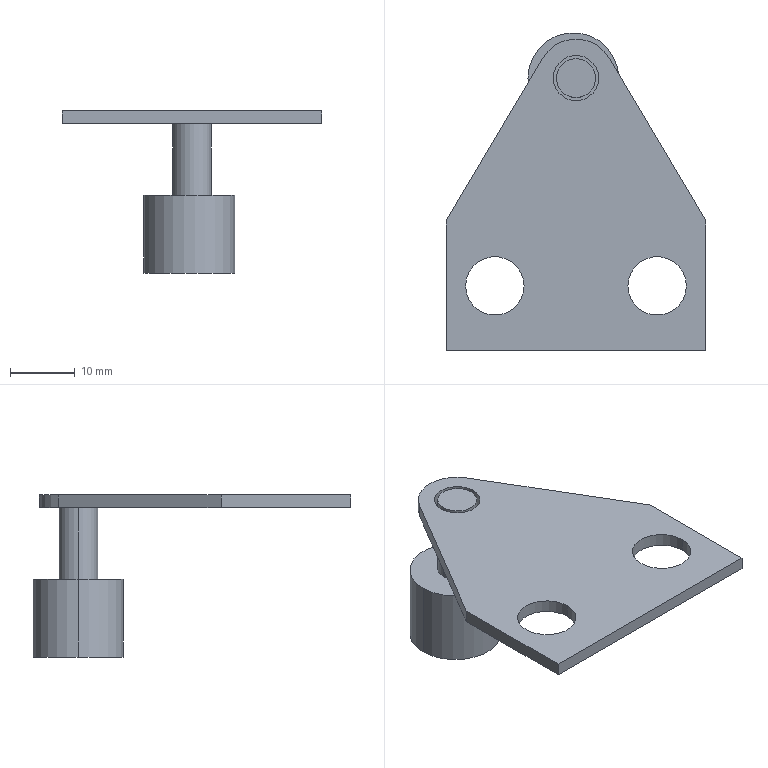Part | SolidWorks | features BaseBody 2 | 2 solids | 21 faces | box 40 x 49 x 25 mm | volume 4787 mm3 | cylinder 11 | plane 10 | commonest cylinder face diameters 9 x4 6 x2 7 x2 14 x2 12 x1
STEP:
#1=CARTESIAN_POINT('',(28.,10.,0.));
#2=VERTEX_POINT('',#1);
#3=CARTESIAN_POINT('',(37.,10.,0.));
#4=VERTEX_POINT('',#3);
#5=CARTESIAN_POINT('',(32.5,10.,0.));
#6=DIRECTION('',(0.,0.,1.));
#7=DIRECTION('',(1.,0.,0.));
#8=AXIS2_PLACEMENT_3D('',#5,#6,#7);
#9=CIRCLE('',#8,4.5);
#10=EDGE_CURVE('',#2,#4,#9,.T.);
#11=ORIENTED_EDGE('',*,*,#10,.F.);
#12=CARTESIAN_POINT('',(28.,10.,2.));
#13=VERTEX_POINT('',#12);
#14=CARTESIAN_POINT('',(28.,10.,0.));
#15=DIRECTION('',(0.,0.,1.));
#16=VECTOR('',#15,1000.);
#17=LINE('',#14,#16);
#18=EDGE_CURVE('',#2,#13,#17,.T.);
#19=ORIENTED_EDGE('',*,*,#18,.T.);
#20=CARTESIAN_POINT('',(37.,10.,2.));
#21=VERTEX_POINT('',#20);
#22=CARTESIAN_POINT('',(32.5,10.,2.));
#23=DIRECTION('',(0.,0.,1.));
#24=DIRECTION('',(1.,0.,0.));
#25=AXIS2_PLACEMENT_3D('',#22,#23,#24);
#26=CIRCLE('',#25,4.5);
#27=EDGE_CURVE('',#13,#21,#26,.T.);
#28=ORIENTED_EDGE('',*,*,#27,.T.);
#29=CARTESIAN_POINT('',(37.,10.,0.));
#30=DIRECTION('',(0.,0.,1.));
#31=VECTOR('',#30,1000.);
#32=LINE('',#29,#31);
#33=EDGE_CURVE('',#4,#21,#32,.T.);
#34=ORIENTED_EDGE('',*,*,#33,.F.);
#35=EDGE_LOOP('',(#11,#19,#28,#34));
#36=FACE_OUTER_BOUND('',#35,.T.);
#37=CARTESIAN_POINT('',(32.5,10.,0.));
#38=DIRECTION('',(0.,0.,1.));
#39=DIRECTION('',(1.,0.,0.));
#40=AXIS2_PLACEMENT_3D('',#37,#38,#39);
#41=CYLINDRICAL_SURFACE('',#40,4.5);
#42=ADVANCED_FACE('',(#36),#41,.F.);
#43=CARTESIAN_POINT('',(3.,10.,0.));
#44=VERTEX_POINT('',#43);
#45=CARTESIAN_POINT('',(12.,10.,0.));
#46=VERTEX_POINT('',#45);
#47=CARTESIAN_POINT('',(7.5,10.,0.));
#48=DIRECTION('',(0.,0.,1.));
#49=DIRECTION('',(1.,0.,0.));
#50=AXIS2_PLACEMENT_3D('',#47,#48,#49);
#51=CIRCLE('',#50,4.5);
#52=EDGE_CURVE('',#44,#46,#51,.T.);
#53=ORIENTED_EDGE('',*,*,#52,.F.);
#54=CARTESIAN_POINT('',(3.,10.,2.));
#55=VERTEX_POINT('',#54);
#56=CARTESIAN_POINT('',(3.,10.,0.));
#57=DIRECTION('',(0.,0.,1.));
#58=VECTOR('',#57,1000.);
#59=LINE('',#56,#58);
#60=EDGE_CURVE('',#44,#55,#59,.T.);
#61=ORIENTED_EDGE('',*,*,#60,.T.);
#62=CARTESIAN_POINT('',(12.,10.,2.));
#63=VERTEX_POINT('',#62);
#64=CARTESIAN_POINT('',(7.5,10.,2.));
#65=DIRECTION('',(0.,0.,1.));
#66=DIRECTION('',(1.,0.,0.));
#67=AXIS2_PLACEMENT_3D('',#64,#65,#66);
#68=CIRCLE('',#67,4.5);
#69=EDGE_CURVE('',#55,#63,#68,.T.);
#70=ORIENTED_EDGE('',*,*,#69,.T.);
#71=CARTESIAN_POINT('',(12.,10.,0.));
#72=DIRECTION('',(0.,0.,1.));
#73=VECTOR('',#72,1000.);
#74=LINE('',#71,#73);
#75=EDGE_CURVE('',#46,#63,#74,.T.);
#76=ORIENTED_EDGE('',*,*,#75,.F.);
#77=EDGE_LOOP('',(#53,#61,#70,#76));
#78=FACE_OUTER_BOUND('',#77,.T.);
#79=CARTESIAN_POINT('',(7.5,10.,0.));
#80=DIRECTION('',(0.,0.,1.));
#81=DIRECTION('',(1.,0.,0.));
#82=AXIS2_PLACEMENT_3D('',#79,#80,#81);
#83=CYLINDRICAL_SURFACE('',#82,4.5);
#84=ADVANCED_FACE('',(#78),#83,.F.);
#85=CARTESIAN_POINT('',(16.5,42.,0.));
#86=VERTEX_POINT('',#85);
#87=CARTESIAN_POINT('',(23.5,42.,0.));
#88=VERTEX_POINT('',#87);
#89=CARTESIAN_POINT('',(20.,42.,0.));
#90=DIRECTION('',(0.,0.,1.));
#91=DIRECTION('',(1.,0.,0.));
#92=AXIS2_PLACEMENT_3D('',#89,#90,#91);
#93=CIRCLE('',#92,3.5);
#94=EDGE_CURVE('',#86,#88,#93,.T.);
#95=ORIENTED_EDGE('',*,*,#94,.F.);
#96=CARTESIAN_POINT('',(16.5,42.,2.));
#97=VERTEX_POINT('',#96);
#98=CARTESIAN_POINT('',(16.5,42.,0.));
#99=DIRECTION('',(0.,0.,1.));
#100=VECTOR('',#99,1000.);
#101=LINE('',#98,#100);
#102=EDGE_CURVE('',#86,#97,#101,.T.);
#103=ORIENTED_EDGE('',*,*,#102,.T.);
#104=CARTESIAN_POINT('',(23.5,42.,2.));
#105=VERTEX_POINT('',#104);
#106=CARTESIAN_POINT('',(20.,42.,2.));
#107=DIRECTION('',(0.,0.,1.));
#108=DIRECTION('',(1.,0.,0.));
#109=AXIS2_PLACEMENT_3D('',#106,#107,#108);
#110=CIRCLE('',#109,3.5);
#111=EDGE_CURVE('',#97,#105,#110,.T.);
#112=ORIENTED_EDGE('',*,*,#111,.T.);
#113=CARTESIAN_POINT('',(23.5,42.,0.));
#114=DIRECTION('',(0.,0.,1.));
#115=VECTOR('',#114,1000.);
#116=LINE('',#113,#115);
#117=EDGE_CURVE('',#88,#105,#116,.T.);
#118=ORIENTED_EDGE('',*,*,#117,.F.);
#119=EDGE_LOOP('',(#95,#103,#112,#118));
#120=FACE_OUTER_BOUND('',#119,.T.);
#121=CARTESIAN_POINT('',(20.,42.,0.));
#122=DIRECTION('',(0.,0.,1.));
#123=DIRECTION('',(1.,0.,0.));
#124=AXIS2_PLACEMENT_3D('',#121,#122,#123);
#125=CYLINDRICAL_SURFACE('',#124,3.5);
#126=ADVANCED_FACE('',(#120),#125,.F.);
#127=CARTESIAN_POINT('',(14.837,45.057,2.));
#128=VERTEX_POINT('',#127);
#129=CARTESIAN_POINT('',(0.,20.,2.));
#130=VERTEX_POINT('',#129);
#131=CARTESIAN_POINT('',(14.837,45.057,2.));
#132=DIRECTION('',(-0.5095,-0.8605,0.));
#133=VECTOR('',#132,1000.);
#134=LINE('',#131,#133);
#135=EDGE_CURVE('',#128,#130,#134,.T.);
#136=ORIENTED_EDGE('',*,*,#135,.F.);
#137=CARTESIAN_POINT('',(14.837,45.057,0.));
#138=VERTEX_POINT('',#137);
#139=CARTESIAN_POINT('',(14.837,45.057,0.));
#140=DIRECTION('',(0.,0.,1.));
#141=VECTOR('',#140,1000.);
#142=LINE('',#139,#141);
#143=EDGE_CURVE('',#138,#128,#142,.T.);
#144=ORIENTED_EDGE('',*,*,#143,.F.);
#145=CARTESIAN_POINT('',(0.,20.,0.));
#146=VERTEX_POINT('',#145);
#147=CARTESIAN_POINT('',(14.837,45.057,0.));
#148=DIRECTION('',(-0.5095,-0.8605,0.));
#149=VECTOR('',#148,1000.);
#150=LINE('',#147,#149);
#151=EDGE_CURVE('',#138,#146,#150,.T.);
#152=ORIENTED_EDGE('',*,*,#151,.T.);
#153=CARTESIAN_POINT('',(0.,20.,0.));
#154=DIRECTION('',(0.,0.,1.));
#155=VECTOR('',#154,1000.);
#156=LINE('',#153,#155);
#157=EDGE_CURVE('',#146,#130,#156,.T.);
#158=ORIENTED_EDGE('',*,*,#157,.T.);
#159=EDGE_LOOP('',(#136,#144,#152,#158));
#160=FACE_OUTER_BOUND('',#159,.T.);
#161=CARTESIAN_POINT('',(14.837,45.057,0.));
#162=DIRECTION('',(-0.8605,0.5095,0.));
#163=DIRECTION('',(0.,0.,1.));
#164=AXIS2_PLACEMENT_3D('',#161,#162,#163);
#165=PLANE('',#164);
#166=ADVANCED_FACE('',(#160),#165,.T.);
#167=CARTESIAN_POINT('',(40.,20.,2.));
#168=VERTEX_POINT('',#167);
#169=CARTESIAN_POINT('',(25.163,45.057,2.));
#170=VERTEX_POINT('',#169);
#171=CARTESIAN_POINT('',(40.,20.,2.));
#172=DIRECTION('',(-0.5095,0.8605,0.));
#173=VECTOR('',#172,1000.);
#174=LINE('',#171,#173);
#175=EDGE_CURVE('',#168,#170,#174,.T.);
#176=ORIENTED_EDGE('',*,*,#175,.F.);
#177=CARTESIAN_POINT('',(40.,20.,0.));
#178=VERTEX_POINT('',#177);
#179=CARTESIAN_POINT('',(40.,20.,0.));
#180=DIRECTION('',(0.,0.,1.));
#181=VECTOR('',#180,1000.);
#182=LINE('',#179,#181);
#183=EDGE_CURVE('',#178,#168,#182,.T.);
#184=ORIENTED_EDGE('',*,*,#183,.F.);
#185=CARTESIAN_POINT('',(25.163,45.057,0.));
#186=VERTEX_POINT('',#185);
#187=CARTESIAN_POINT('',(40.,20.,0.));
#188=DIRECTION('',(-0.5095,0.8605,0.));
#189=VECTOR('',#188,1000.);
#190=LINE('',#187,#189);
#191=EDGE_CURVE('',#178,#186,#190,.T.);
#192=ORIENTED_EDGE('',*,*,#191,.T.);
#193=CARTESIAN_POINT('',(25.163,45.057,0.));
#194=DIRECTION('',(0.,0.,1.));
#195=VECTOR('',#194,1000.);
#196=LINE('',#193,#195);
#197=EDGE_CURVE('',#186,#170,#196,.T.);
#198=ORIENTED_EDGE('',*,*,#197,.T.);
#199=EDGE_LOOP('',(#176,#184,#192,#198));
#200=FACE_OUTER_BOUND('',#199,.T.);
#201=CARTESIAN_POINT('',(40.,20.,0.));
#202=DIRECTION('',(0.8605,0.5095,0.));
#203=DIRECTION('',(0.,0.,-1.));
#204=AXIS2_PLACEMENT_3D('',#201,#202,#203);
#205=PLANE('',#204);
#206=ADVANCED_FACE('',(#200),#205,.T.);
#207=ORIENTED_EDGE('',*,*,#197,.F.);
#208=CARTESIAN_POINT('',(20.,42.,0.));
#209=DIRECTION('',(0.,0.,-1.));
#210=DIRECTION('',(-1.,0.,0.));
#211=AXIS2_PLACEMENT_3D('',#208,#209,#210);
#212=CIRCLE('',#211,6.);
#213=EDGE_CURVE('',#138,#186,#212,.T.);
#214=ORIENTED_EDGE('',*,*,#213,.F.);
#215=ORIENTED_EDGE('',*,*,#143,.T.);
#216=CARTESIAN_POINT('',(20.,42.,2.));
#217=DIRECTION('',(0.,0.,1.));
#218=DIRECTION('',(1.,0.,0.));
#219=AXIS2_PLACEMENT_3D('',#216,#217,#218);
#220=CIRCLE('',#219,6.);
#221=EDGE_CURVE('',#170,#128,#220,.T.);
#222=ORIENTED_EDGE('',*,*,#221,.F.);
#223=EDGE_LOOP('',(#207,#214,#215,#222));
#224=FACE_OUTER_BOUND('',#223,.T.);
#225=CARTESIAN_POINT('',(20.,42.,0.));
#226=DIRECTION('',(0.,0.,1.));
#227=DIRECTION('',(1.,0.,0.));
#228=AXIS2_PLACEMENT_3D('',#225,#226,#227);
#229=CYLINDRICAL_SURFACE('',#228,6.);
#230=ADVANCED_FACE('',(#224),#229,.T.);
#231=CARTESIAN_POINT('',(0.,0.,0.));
#232=VERTEX_POINT('',#231);
#233=CARTESIAN_POINT('',(40.,0.,0.));
#234=VERTEX_POINT('',#233);
#235=CARTESIAN_POINT('',(0.,0.,0.));
#236=DIRECTION('',(1.,0.,0.));
#237=VECTOR('',#236,1000.);
#238=LINE('',#235,#237);
#239=EDGE_CURVE('',#232,#234,#238,.T.);
#240=ORIENTED_EDGE('',*,*,#239,.T.);
#241=CARTESIAN_POINT('',(40.,0.,2.));
#242=VERTEX_POINT('',#241);
#243=CARTESIAN_POINT('',(40.,0.,2.));
#244=DIRECTION('',(0.,0.,-1.));
#245=VECTOR('',#244,1000.);
#246=LINE('',#243,#245);
#247=EDGE_CURVE('',#242,#234,#246,.T.);
#248=ORIENTED_EDGE('',*,*,#247,.F.);
#249=CARTESIAN_POINT('',(0.,0.,2.));
#250=VERTEX_POINT('',#249);
#251=CARTESIAN_POINT('',(0.,0.,2.));
#252=DIRECTION('',(1.,0.,0.));
#253=VECTOR('',#252,1000.);
#254=LINE('',#251,#253);
#255=EDGE_CURVE('',#250,#242,#254,.T.);
#256=ORIENTED_EDGE('',*,*,#255,.F.);
#257=CARTESIAN_POINT('',(0.,0.,2.));
#258=DIRECTION('',(0.,0.,-1.));
#259=VECTOR('',#258,1000.);
#260=LINE('',#257,#259);
#261=EDGE_CURVE('',#250,#232,#260,.T.);
#262=ORIENTED_EDGE('',*,*,#261,.T.);
#263=EDGE_LOOP('',(#240,#248,#256,#262));
#264=FACE_OUTER_BOUND('',#263,.T.);
#265=CARTESIAN_POINT('',(0.,0.,2.));
#266=DIRECTION('',(0.,1.,0.));
#267=DIRECTION('',(1.,0.,0.));
#268=AXIS2_PLACEMENT_3D('',#265,#266,#267);
#269=PLANE('',#268);
#270=ADVANCED_FACE('',(#264),#269,.F.);
#271=CARTESIAN_POINT('',(20.,42.,0.));
#272=DIRECTION('',(0.,0.,1.));
#273=DIRECTION('',(1.,0.,0.));
#274=AXIS2_PLACEMENT_3D('',#271,#272,#273);
#275=CIRCLE('',#274,3.5);
#276=EDGE_CURVE('',#88,#86,#275,.T.);
#277=ORIENTED_EDGE('',*,*,#276,.T.);
#278=ORIENTED_EDGE('',*,*,#94,.T.);
#279=EDGE_LOOP('',(#277,#278));
#280=FACE_BOUND('',#279,.T.);
#281=CARTESIAN_POINT('',(7.5,10.,0.));
#282=DIRECTION('',(0.,0.,1.));
#283=DIRECTION('',(1.,0.,0.));
#284=AXIS2_PLACEMENT_3D('',#281,#282,#283);
#285=CIRCLE('',#284,4.5);
#286=EDGE_CURVE('',#46,#44,#285,.T.);
#287=ORIENTED_EDGE('',*,*,#286,.T.);
#288=ORIENTED_EDGE('',*,*,#52,.T.);
#289=EDGE_LOOP('',(#287,#288));
#290=FACE_BOUND('',#289,.T.);
#291=CARTESIAN_POINT('',(32.5,10.,0.));
#292=DIRECTION('',(0.,0.,1.));
#293=DIRECTION('',(1.,0.,0.));
#294=AXIS2_PLACEMENT_3D('',#291,#292,#293);
#295=CIRCLE('',#294,4.5);
#296=EDGE_CURVE('',#4,#2,#295,.T.);
#297=ORIENTED_EDGE('',*,*,#296,.T.);
#298=ORIENTED_EDGE('',*,*,#10,.T.);
#299=EDGE_LOOP('',(#297,#298));
#300=FACE_BOUND('',#299,.T.);
#301=ORIENTED_EDGE('',*,*,#213,.T.);
#302=ORIENTED_EDGE('',*,*,#191,.F.);
#303=CARTESIAN_POINT('',(40.,0.,0.));
#304=DIRECTION('',(0.,1.,0.));
#305=VECTOR('',#304,1000.);
#306=LINE('',#303,#305);
#307=EDGE_CURVE('',#234,#178,#306,.T.);
#308=ORIENTED_EDGE('',*,*,#307,.F.);
#309=ORIENTED_EDGE('',*,*,#239,.F.);
#310=CARTESIAN_POINT('',(0.,0.,0.));
#311=DIRECTION('',(0.,-1.,0.));
#312=VECTOR('',#311,1000.);
#313=LINE('',#310,#312);
#314=EDGE_CURVE('',#146,#232,#313,.T.);
#315=ORIENTED_EDGE('',*,*,#314,.F.);
#316=ORIENTED_EDGE('',*,*,#151,.F.);
#317=EDGE_LOOP('',(#301,#302,#308,#309,#315,#316));
#318=FACE_OUTER_BOUND('',#317,.T.);
#319=CARTESIAN_POINT('',(0.,0.,0.));
#320=DIRECTION('',(0.,0.,-1.));
#321=DIRECTION('',(0.,-1.,0.));
#322=AXIS2_PLACEMENT_3D('',#319,#320,#321);
#323=PLANE('',#322);
#324=ADVANCED_FACE('',(#280,#290,#300,#318),#323,.T.);
#325=CARTESIAN_POINT('',(20.,42.,2.));
#326=DIRECTION('',(0.,0.,1.));
#327=DIRECTION('',(1.,0.,0.));
#328=AXIS2_PLACEMENT_3D('',#325,#326,#327);
#329=CIRCLE('',#328,3.5);
#330=EDGE_CURVE('',#105,#97,#329,.T.);
#331=ORIENTED_EDGE('',*,*,#330,.F.);
#332=ORIENTED_EDGE('',*,*,#111,.F.);
#333=EDGE_LOOP('',(#331,#332));
#334=FACE_BOUND('',#333,.T.);
#335=CARTESIAN_POINT('',(7.5,10.,2.));
#336=DIRECTION('',(0.,0.,1.));
#337=DIRECTION('',(1.,0.,0.));
#338=AXIS2_PLACEMENT_3D('',#335,#336,#337);
#339=CIRCLE('',#338,4.5);
#340=EDGE_CURVE('',#63,#55,#339,.T.);
#341=ORIENTED_EDGE('',*,*,#340,.F.);
#342=ORIENTED_EDGE('',*,*,#69,.F.);
#343=EDGE_LOOP('',(#341,#342));
#344=FACE_BOUND('',#343,.T.);
#345=CARTESIAN_POINT('',(32.5,10.,2.));
#346=DIRECTION('',(0.,0.,1.));
#347=DIRECTION('',(1.,0.,0.));
#348=AXIS2_PLACEMENT_3D('',#345,#346,#347);
#349=CIRCLE('',#348,4.5);
#350=EDGE_CURVE('',#21,#13,#349,.T.);
#351=ORIENTED_EDGE('',*,*,#350,.F.);
#352=ORIENTED_EDGE('',*,*,#27,.F.);
#353=EDGE_LOOP('',(#351,#352));
#354=FACE_BOUND('',#353,.T.);
#355=ORIENTED_EDGE('',*,*,#175,.T.);
#356=ORIENTED_EDGE('',*,*,#221,.T.);
#357=ORIENTED_EDGE('',*,*,#135,.T.);
#358=CARTESIAN_POINT('',(0.,0.,2.));
#359=DIRECTION('',(0.,-1.,0.));
#360=VECTOR('',#359,1000.);
#361=LINE('',#358,#360);
#362=EDGE_CURVE('',#130,#250,#361,.T.);
#363=ORIENTED_EDGE('',*,*,#362,.T.);
#364=ORIENTED_EDGE('',*,*,#255,.T.);
#365=CARTESIAN_POINT('',(40.,0.,2.));
#366=DIRECTION('',(0.,1.,0.));
#367=VECTOR('',#366,1000.);
#368=LINE('',#365,#367);
#369=EDGE_CURVE('',#242,#168,#368,.T.);
#370=ORIENTED_EDGE('',*,*,#369,.T.);
#371=EDGE_LOOP('',(#355,#356,#357,#363,#364,#370));
#372=FACE_OUTER_BOUND('',#371,.T.);
#373=CARTESIAN_POINT('',(0.,0.,2.));
#374=DIRECTION('',(0.,0.,-1.));
#375=DIRECTION('',(0.,-1.,0.));
#376=AXIS2_PLACEMENT_3D('',#373,#374,#375);
#377=PLANE('',#376);
#378=ADVANCED_FACE('',(#334,#344,#354,#372),#377,.F.);
#379=ORIENTED_EDGE('',*,*,#183,.T.);
#380=ORIENTED_EDGE('',*,*,#369,.F.);
#381=ORIENTED_EDGE('',*,*,#247,.T.);
#382=ORIENTED_EDGE('',*,*,#307,.T.);
#383=EDGE_LOOP('',(#379,#380,#381,#382));
#384=FACE_OUTER_BOUND('',#383,.T.);
#385=CARTESIAN_POINT('',(40.,0.,2.));
#386=DIRECTION('',(-1.,0.,0.));
#387=DIRECTION('',(0.,0.,1.));
#388=AXIS2_PLACEMENT_3D('',#385,#386,#387);
#389=PLANE('',#388);
#390=ADVANCED_FACE('',(#384),#389,.F.);
#391=ORIENTED_EDGE('',*,*,#157,.F.);
#392=ORIENTED_EDGE('',*,*,#314,.T.);
#393=ORIENTED_EDGE('',*,*,#261,.F.);
#394=ORIENTED_EDGE('',*,*,#362,.F.);
#395=EDGE_LOOP('',(#391,#392,#393,#394));
#396=FACE_OUTER_BOUND('',#395,.T.);
#397=CARTESIAN_POINT('',(0.,0.,2.));
#398=DIRECTION('',(1.,0.,0.));
#399=DIRECTION('',(0.,1.,0.));
#400=AXIS2_PLACEMENT_3D('',#397,#398,#399);
#401=PLANE('',#400);
#402=ADVANCED_FACE('',(#396),#401,.F.);
#403=ORIENTED_EDGE('',*,*,#102,.F.);
#404=ORIENTED_EDGE('',*,*,#276,.F.);
#405=ORIENTED_EDGE('',*,*,#117,.T.);
#406=ORIENTED_EDGE('',*,*,#330,.T.);
#407=EDGE_LOOP('',(#403,#404,#405,#406));
#408=FACE_OUTER_BOUND('',#407,.T.);
#409=CARTESIAN_POINT('',(20.,42.,0.));
#410=DIRECTION('',(0.,0.,1.));
#411=DIRECTION('',(1.,0.,0.));
#412=AXIS2_PLACEMENT_3D('',#409,#410,#411);
#413=CYLINDRICAL_SURFACE('',#412,3.5);
#414=ADVANCED_FACE('',(#408),#413,.F.);
#415=ORIENTED_EDGE('',*,*,#60,.F.);
#416=ORIENTED_EDGE('',*,*,#286,.F.);
#417=ORIENTED_EDGE('',*,*,#75,.T.);
#418=ORIENTED_EDGE('',*,*,#340,.T.);
#419=EDGE_LOOP('',(#415,#416,#417,#418));
#420=FACE_OUTER_BOUND('',#419,.T.);
#421=CARTESIAN_POINT('',(7.5,10.,0.));
#422=DIRECTION('',(0.,0.,1.));
#423=DIRECTION('',(1.,0.,0.));
#424=AXIS2_PLACEMENT_3D('',#421,#422,#423);
#425=CYLINDRICAL_SURFACE('',#424,4.5);
#426=ADVANCED_FACE('',(#420),#425,.F.);
#427=ORIENTED_EDGE('',*,*,#18,.F.);
#428=ORIENTED_EDGE('',*,*,#296,.F.);
#429=ORIENTED_EDGE('',*,*,#33,.T.);
#430=ORIENTED_EDGE('',*,*,#350,.T.);
#431=EDGE_LOOP('',(#427,#428,#429,#430));
#432=FACE_OUTER_BOUND('',#431,.T.);
#433=CARTESIAN_POINT('',(32.5,10.,0.));
#434=DIRECTION('',(0.,0.,1.));
#435=DIRECTION('',(1.,0.,0.));
#436=AXIS2_PLACEMENT_3D('',#433,#434,#435);
#437=CYLINDRICAL_SURFACE('',#436,4.5);
#438=ADVANCED_FACE('',(#432),#437,.F.);
#439=CLOSED_SHELL('',(#42,#84,#126,#166,#206,#230,#270,#324,#378,#390,#402,#414,#426,#438));
#440=MANIFOLD_SOLID_BREP('',#439);
#441=CARTESIAN_POINT('',(12.592,42.,-23.));
#442=VERTEX_POINT('',#441);
#443=CARTESIAN_POINT('',(26.592,42.,-23.));
#444=VERTEX_POINT('',#443);
#445=CARTESIAN_POINT('',(19.592,42.,-23.));
#446=DIRECTION('',(0.,0.,-1.));
#447=DIRECTION('',(-1.,0.,0.));
#448=AXIS2_PLACEMENT_3D('',#445,#446,#447);
#449=CIRCLE('',#448,7.);
#450=EDGE_CURVE('',#442,#444,#449,.T.);
#451=ORIENTED_EDGE('',*,*,#450,.F.);
#452=CARTESIAN_POINT('',(12.592,42.,-11.));
#453=VERTEX_POINT('',#452);
#454=CARTESIAN_POINT('',(12.592,42.,-23.));
#455=DIRECTION('',(0.,0.,1.));
#456=VECTOR('',#455,1000.);
#457=LINE('',#454,#456);
#458=EDGE_CURVE('',#442,#453,#457,.T.);
#459=ORIENTED_EDGE('',*,*,#458,.T.);
#460=CARTESIAN_POINT('',(26.592,42.,-11.));
#461=VERTEX_POINT('',#460);
#462=CARTESIAN_POINT('',(19.592,42.,-11.));
#463=DIRECTION('',(0.,0.,-1.));
#464=DIRECTION('',(-1.,0.,0.));
#465=AXIS2_PLACEMENT_3D('',#462,#463,#464);
#466=CIRCLE('',#465,7.);
#467=EDGE_CURVE('',#453,#461,#466,.T.);
#468=ORIENTED_EDGE('',*,*,#467,.T.);
#469=CARTESIAN_POINT('',(26.592,42.,-23.));
#470=DIRECTION('',(0.,0.,1.));
#471=VECTOR('',#470,1000.);
#472=LINE('',#469,#471);
#473=EDGE_CURVE('',#444,#461,#472,.T.);
#474=ORIENTED_EDGE('',*,*,#473,.F.);
#475=EDGE_LOOP('',(#451,#459,#468,#474));
#476=FACE_OUTER_BOUND('',#475,.T.);
#477=CARTESIAN_POINT('',(19.592,42.,-23.));
#478=DIRECTION('',(0.,0.,1.));
#479=DIRECTION('',(1.,0.,0.));
#480=AXIS2_PLACEMENT_3D('',#477,#478,#479);
#481=CYLINDRICAL_SURFACE('',#480,7.);
#482=ADVANCED_FACE('',(#476),#481,.T.);
#483=CARTESIAN_POINT('',(23.,42.,-11.));
#484=VERTEX_POINT('',#483);
#485=CARTESIAN_POINT('',(17.,42.,-11.));
#486=VERTEX_POINT('',#485);
#487=CARTESIAN_POINT('',(20.,42.,-11.));
#488=DIRECTION('',(0.,0.,1.));
#489=DIRECTION('',(-1.,0.,0.));
#490=AXIS2_PLACEMENT_3D('',#487,#488,#489);
#491=CIRCLE('',#490,3.);
#492=EDGE_CURVE('',#484,#486,#491,.T.);
#493=ORIENTED_EDGE('',*,*,#492,.T.);
#494=CARTESIAN_POINT('',(17.,42.,2.));
#495=VERTEX_POINT('',#494);
#496=CARTESIAN_POINT('',(17.,42.,-11.));
#497=DIRECTION('',(0.,0.,1.));
#498=VECTOR('',#497,1000.);
#499=LINE('',#496,#498);
#500=EDGE_CURVE('',#486,#495,#499,.T.);
#501=ORIENTED_EDGE('',*,*,#500,.T.);
#502=CARTESIAN_POINT('',(23.,42.,2.));
#503=VERTEX_POINT('',#502);
#504=CARTESIAN_POINT('',(20.,42.,2.));
#505=DIRECTION('',(0.,0.,1.));
#506=DIRECTION('',(1.,0.,0.));
#507=AXIS2_PLACEMENT_3D('',#504,#505,#506);
#508=CIRCLE('',#507,3.);
#509=EDGE_CURVE('',#503,#495,#508,.T.);
#510=ORIENTED_EDGE('',*,*,#509,.F.);
#511=CARTESIAN_POINT('',(23.,42.,-11.));
#512=DIRECTION('',(0.,0.,1.));
#513=VECTOR('',#512,1000.);
#514=LINE('',#511,#513);
#515=EDGE_CURVE('',#484,#503,#514,.T.);
#516=ORIENTED_EDGE('',*,*,#515,.F.);
#517=EDGE_LOOP('',(#493,#501,#510,#516));
#518=FACE_OUTER_BOUND('',#517,.T.);
#519=CARTESIAN_POINT('',(20.,42.,-11.));
#520=DIRECTION('',(0.,0.,1.));
#521=DIRECTION('',(1.,0.,0.));
#522=AXIS2_PLACEMENT_3D('',#519,#520,#521);
#523=CYLINDRICAL_SURFACE('',#522,3.);
#524=ADVANCED_FACE('',(#518),#523,.T.);
#525=ORIENTED_EDGE('',*,*,#492,.F.);
#526=CARTESIAN_POINT('',(20.,42.,-11.));
#527=DIRECTION('',(0.,0.,1.));
#528=DIRECTION('',(-1.,0.,0.));
#529=AXIS2_PLACEMENT_3D('',#526,#527,#528);
#530=CIRCLE('',#529,3.);
#531=EDGE_CURVE('',#486,#484,#530,.T.);
#532=ORIENTED_EDGE('',*,*,#531,.F.);
#533=EDGE_LOOP('',(#525,#532));
#534=FACE_BOUND('',#533,.T.);
#535=CARTESIAN_POINT('',(19.592,42.,-11.));
#536=DIRECTION('',(0.,0.,-1.));
#537=DIRECTION('',(-1.,0.,0.));
#538=AXIS2_PLACEMENT_3D('',#535,#536,#537);
#539=CIRCLE('',#538,7.);
#540=EDGE_CURVE('',#461,#453,#539,.T.);
#541=ORIENTED_EDGE('',*,*,#540,.F.);
#542=ORIENTED_EDGE('',*,*,#467,.F.);
#543=EDGE_LOOP('',(#541,#542));
#544=FACE_OUTER_BOUND('',#543,.T.);
#545=CARTESIAN_POINT('',(19.592,42.,-11.));
#546=DIRECTION('',(0.,0.,-1.));
#547=DIRECTION('',(0.,-1.,0.));
#548=AXIS2_PLACEMENT_3D('',#545,#546,#547);
#549=PLANE('',#548);
#550=ADVANCED_FACE('',(#534,#544),#549,.F.);
#551=CARTESIAN_POINT('',(19.592,42.,-23.));
#552=DIRECTION('',(0.,0.,-1.));
#553=DIRECTION('',(-1.,0.,0.));
#554=AXIS2_PLACEMENT_3D('',#551,#552,#553);
#555=CIRCLE('',#554,7.);
#556=EDGE_CURVE('',#444,#442,#555,.T.);
#557=ORIENTED_EDGE('',*,*,#556,.T.);
#558=ORIENTED_EDGE('',*,*,#450,.T.);
#559=EDGE_LOOP('',(#557,#558));
#560=FACE_OUTER_BOUND('',#559,.T.);
#561=CARTESIAN_POINT('',(19.592,42.,-23.));
#562=DIRECTION('',(0.,0.,-1.));
#563=DIRECTION('',(0.,-1.,0.));
#564=AXIS2_PLACEMENT_3D('',#561,#562,#563);
#565=PLANE('',#564);
#566=ADVANCED_FACE('',(#560),#565,.T.);
#567=ORIENTED_EDGE('',*,*,#509,.T.);
#568=CARTESIAN_POINT('',(20.,42.,2.));
#569=DIRECTION('',(0.,0.,1.));
#570=DIRECTION('',(1.,0.,0.));
#571=AXIS2_PLACEMENT_3D('',#568,#569,#570);
#572=CIRCLE('',#571,3.);
#573=EDGE_CURVE('',#495,#503,#572,.T.);
#574=ORIENTED_EDGE('',*,*,#573,.T.);
#575=EDGE_LOOP('',(#567,#574));
#576=FACE_OUTER_BOUND('',#575,.T.);
#577=CARTESIAN_POINT('',(20.,42.,2.));
#578=DIRECTION('',(0.,0.,1.));
#579=DIRECTION('',(1.,0.,0.));
#580=AXIS2_PLACEMENT_3D('',#577,#578,#579);
#581=PLANE('',#580);
#582=ADVANCED_FACE('',(#576),#581,.T.);
#583=ORIENTED_EDGE('',*,*,#500,.F.);
#584=ORIENTED_EDGE('',*,*,#531,.T.);
#585=ORIENTED_EDGE('',*,*,#515,.T.);
#586=ORIENTED_EDGE('',*,*,#573,.F.);
#587=EDGE_LOOP('',(#583,#584,#585,#586));
#588=FACE_OUTER_BOUND('',#587,.T.);
#589=CARTESIAN_POINT('',(20.,42.,-11.));
#590=DIRECTION('',(0.,0.,1.));
#591=DIRECTION('',(1.,0.,0.));
#592=AXIS2_PLACEMENT_3D('',#589,#590,#591);
#593=CYLINDRICAL_SURFACE('',#592,3.);
#594=ADVANCED_FACE('',(#588),#593,.T.);
#595=ORIENTED_EDGE('',*,*,#458,.F.);
#596=ORIENTED_EDGE('',*,*,#556,.F.);
#597=ORIENTED_EDGE('',*,*,#473,.T.);
#598=ORIENTED_EDGE('',*,*,#540,.T.);
#599=EDGE_LOOP('',(#595,#596,#597,#598));
#600=FACE_OUTER_BOUND('',#599,.T.);
#601=CARTESIAN_POINT('',(19.592,42.,-23.));
#602=DIRECTION('',(0.,0.,1.));
#603=DIRECTION('',(1.,0.,0.));
#604=AXIS2_PLACEMENT_3D('',#601,#602,#603);
#605=CYLINDRICAL_SURFACE('',#604,7.);
#606=ADVANCED_FACE('',(#600),#605,.T.);
#607=CLOSED_SHELL('',(#482,#524,#550,#566,#582,#594,#606));
#608=MANIFOLD_SOLID_BREP('',#607);
#609=CARTESIAN_POINT('',(0.,0.,0.));
#610=DIRECTION('',(0.,0.,1.));
#611=DIRECTION('',(1.,0.,0.));
#612=AXIS2_PLACEMENT_3D('',#609,#610,#611);
#613=(LENGTH_UNIT()NAMED_UNIT(*)SI_UNIT(.MILLI.,.METRE.));
#614=UNCERTAINTY_MEASURE_WITH_UNIT(LENGTH_MEASURE(0.00001),#613,'','');
#615=(NAMED_UNIT(*)PLANE_ANGLE_UNIT()SI_UNIT($,.RADIAN.));
#616=(NAMED_UNIT(*)SI_UNIT($,.STERADIAN.)SOLID_ANGLE_UNIT());
#617=(GEOMETRIC_REPRESENTATION_CONTEXT(3)GLOBAL_UNCERTAINTY_ASSIGNED_CONTEXT((#614))GLOBAL_UNIT_ASSIGNED_CONTEXT((#613,#615,#616))REPRESENTATION_CONTEXT('',''));
#618=ADVANCED_BREP_SHAPE_REPRESENTATION('',(#440,#608,#612),#617);